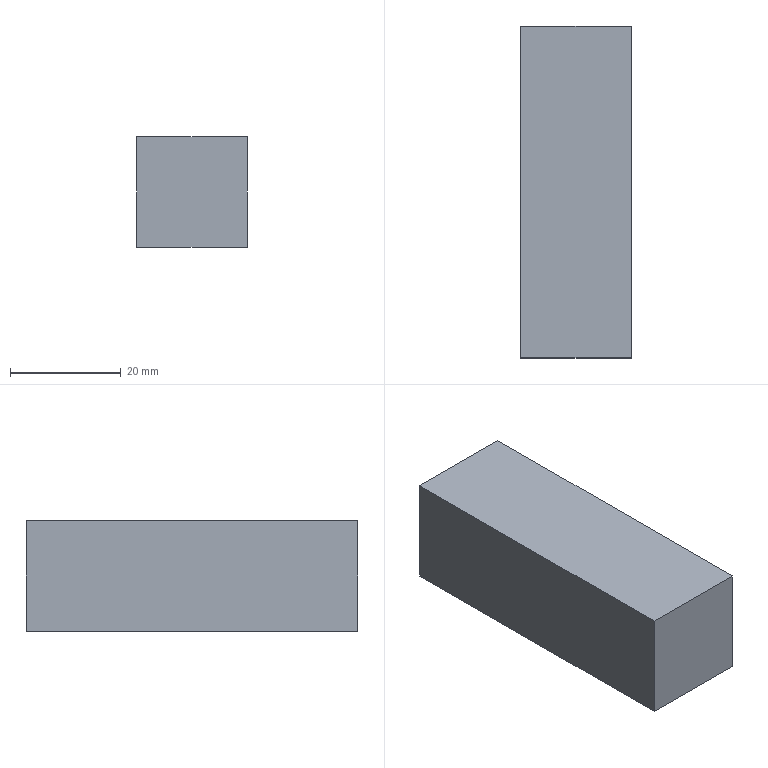Part | STEP file | 冲床-300配套压波_id186_x_t | 1 solid | 6 faces | box 20 x 60 x 20 mm | volume 24000 mm3 | plane 6
STEP:
#1=CARTESIAN_POINT('',(1125.,-215.,0.));
#2=VERTEX_POINT('',#1);
#3=CARTESIAN_POINT('',(1105.,-215.,0.));
#4=VERTEX_POINT('',#3);
#5=CARTESIAN_POINT('',(1105.,-215.,0.));
#6=DIRECTION('',(-1.,0.,0.));
#7=VECTOR('',#6,1.);
#8=LINE('',#5,#7);
#9=EDGE_CURVE('',#2,#4,#8,.T.);
#10=ORIENTED_EDGE('',*,*,#9,.F.);
#11=CARTESIAN_POINT('',(1125.,-155.,0.));
#12=VERTEX_POINT('',#11);
#13=CARTESIAN_POINT('',(1125.,-215.,0.));
#14=DIRECTION('',(0.,-1.,0.));
#15=VECTOR('',#14,1.);
#16=LINE('',#13,#15);
#17=EDGE_CURVE('',#12,#2,#16,.T.);
#18=ORIENTED_EDGE('',*,*,#17,.F.);
#19=CARTESIAN_POINT('',(1105.,-155.,0.));
#20=VERTEX_POINT('',#19);
#21=CARTESIAN_POINT('',(1105.,-155.,0.));
#22=DIRECTION('',(-1.,0.,0.));
#23=VECTOR('',#22,1.);
#24=LINE('',#21,#23);
#25=EDGE_CURVE('',#12,#20,#24,.T.);
#26=ORIENTED_EDGE('',*,*,#25,.T.);
#27=CARTESIAN_POINT('',(1105.,-215.,0.));
#28=DIRECTION('',(0.,-1.,0.));
#29=VECTOR('',#28,1.);
#30=LINE('',#27,#29);
#31=EDGE_CURVE('',#20,#4,#30,.T.);
#32=ORIENTED_EDGE('',*,*,#31,.T.);
#33=EDGE_LOOP('',(#10,#18,#26,#32));
#34=FACE_OUTER_BOUND('',#33,.T.);
#35=CARTESIAN_POINT('',(1105.,-215.,0.));
#36=DIRECTION('',(0.,0.,1.));
#37=DIRECTION('',(0.,1.,0.));
#38=AXIS2_PLACEMENT_3D('',#35,#36,#37);
#39=PLANE('',#38);
#40=ADVANCED_FACE('',(#34),#39,.T.);
#41=ORIENTED_EDGE('',*,*,#25,.F.);
#42=CARTESIAN_POINT('',(1125.,-155.,-20.));
#43=VERTEX_POINT('',#42);
#44=CARTESIAN_POINT('',(1125.,-155.,0.));
#45=DIRECTION('',(0.,0.,1.));
#46=VECTOR('',#45,1.);
#47=LINE('',#44,#46);
#48=EDGE_CURVE('',#43,#12,#47,.T.);
#49=ORIENTED_EDGE('',*,*,#48,.F.);
#50=CARTESIAN_POINT('',(1105.,-155.,-20.));
#51=VERTEX_POINT('',#50);
#52=CARTESIAN_POINT('',(1105.,-155.,-20.));
#53=DIRECTION('',(-1.,0.,0.));
#54=VECTOR('',#53,1.);
#55=LINE('',#52,#54);
#56=EDGE_CURVE('',#43,#51,#55,.T.);
#57=ORIENTED_EDGE('',*,*,#56,.T.);
#58=CARTESIAN_POINT('',(1105.,-155.,0.));
#59=DIRECTION('',(0.,0.,1.));
#60=VECTOR('',#59,1.);
#61=LINE('',#58,#60);
#62=EDGE_CURVE('',#51,#20,#61,.T.);
#63=ORIENTED_EDGE('',*,*,#62,.T.);
#64=EDGE_LOOP('',(#41,#49,#57,#63));
#65=FACE_OUTER_BOUND('',#64,.T.);
#66=CARTESIAN_POINT('',(1105.,-155.,0.));
#67=DIRECTION('',(0.,1.,0.));
#68=DIRECTION('',(0.,0.,-1.));
#69=AXIS2_PLACEMENT_3D('',#66,#67,#68);
#70=PLANE('',#69);
#71=ADVANCED_FACE('',(#65),#70,.T.);
#72=ORIENTED_EDGE('',*,*,#56,.F.);
#73=CARTESIAN_POINT('',(1125.,-215.,-20.));
#74=VERTEX_POINT('',#73);
#75=CARTESIAN_POINT('',(1125.,-215.,-20.));
#76=DIRECTION('',(0.,-1.,0.));
#77=VECTOR('',#76,1.);
#78=LINE('',#75,#77);
#79=EDGE_CURVE('',#43,#74,#78,.T.);
#80=ORIENTED_EDGE('',*,*,#79,.T.);
#81=CARTESIAN_POINT('',(1105.,-215.,-20.));
#82=VERTEX_POINT('',#81);
#83=CARTESIAN_POINT('',(1105.,-215.,-20.));
#84=DIRECTION('',(-1.,0.,0.));
#85=VECTOR('',#84,1.);
#86=LINE('',#83,#85);
#87=EDGE_CURVE('',#74,#82,#86,.T.);
#88=ORIENTED_EDGE('',*,*,#87,.T.);
#89=CARTESIAN_POINT('',(1105.,-215.,-20.));
#90=DIRECTION('',(0.,-1.,0.));
#91=VECTOR('',#90,1.);
#92=LINE('',#89,#91);
#93=EDGE_CURVE('',#51,#82,#92,.T.);
#94=ORIENTED_EDGE('',*,*,#93,.F.);
#95=EDGE_LOOP('',(#72,#80,#88,#94));
#96=FACE_OUTER_BOUND('',#95,.T.);
#97=CARTESIAN_POINT('',(1105.,-215.,-20.));
#98=DIRECTION('',(0.,0.,1.));
#99=DIRECTION('',(0.,1.,0.));
#100=AXIS2_PLACEMENT_3D('',#97,#98,#99);
#101=PLANE('',#100);
#102=ADVANCED_FACE('',(#96),#101,.F.);
#103=CARTESIAN_POINT('',(1105.,-215.,0.));
#104=DIRECTION('',(0.,0.,1.));
#105=VECTOR('',#104,1.);
#106=LINE('',#103,#105);
#107=EDGE_CURVE('',#82,#4,#106,.T.);
#108=ORIENTED_EDGE('',*,*,#107,.F.);
#109=ORIENTED_EDGE('',*,*,#87,.F.);
#110=CARTESIAN_POINT('',(1125.,-215.,0.));
#111=DIRECTION('',(0.,0.,1.));
#112=VECTOR('',#111,1.);
#113=LINE('',#110,#112);
#114=EDGE_CURVE('',#74,#2,#113,.T.);
#115=ORIENTED_EDGE('',*,*,#114,.T.);
#116=ORIENTED_EDGE('',*,*,#9,.T.);
#117=EDGE_LOOP('',(#108,#109,#115,#116));
#118=FACE_OUTER_BOUND('',#117,.T.);
#119=CARTESIAN_POINT('',(1105.,-215.,0.));
#120=DIRECTION('',(0.,1.,0.));
#121=DIRECTION('',(0.,0.,-1.));
#122=AXIS2_PLACEMENT_3D('',#119,#120,#121);
#123=PLANE('',#122);
#124=ADVANCED_FACE('',(#118),#123,.F.);
#125=ORIENTED_EDGE('',*,*,#79,.F.);
#126=ORIENTED_EDGE('',*,*,#48,.T.);
#127=ORIENTED_EDGE('',*,*,#17,.T.);
#128=ORIENTED_EDGE('',*,*,#114,.F.);
#129=EDGE_LOOP('',(#125,#126,#127,#128));
#130=FACE_OUTER_BOUND('',#129,.T.);
#131=CARTESIAN_POINT('',(1125.,-215.,0.));
#132=DIRECTION('',(1.,0.,0.));
#133=DIRECTION('',(0.,0.,-1.));
#134=AXIS2_PLACEMENT_3D('',#131,#132,#133);
#135=PLANE('',#134);
#136=ADVANCED_FACE('',(#130),#135,.T.);
#137=ORIENTED_EDGE('',*,*,#93,.T.);
#138=ORIENTED_EDGE('',*,*,#107,.T.);
#139=ORIENTED_EDGE('',*,*,#31,.F.);
#140=ORIENTED_EDGE('',*,*,#62,.F.);
#141=EDGE_LOOP('',(#137,#138,#139,#140));
#142=FACE_OUTER_BOUND('',#141,.T.);
#143=CARTESIAN_POINT('',(1105.,-215.,0.));
#144=DIRECTION('',(1.,0.,0.));
#145=DIRECTION('',(0.,0.,-1.));
#146=AXIS2_PLACEMENT_3D('',#143,#144,#145);
#147=PLANE('',#146);
#148=ADVANCED_FACE('',(#142),#147,.F.);
#149=CLOSED_SHELL('',(#40,#71,#102,#124,#136,#148));
#150=MANIFOLD_SOLID_BREP('',#149);
#151=(LENGTH_UNIT()NAMED_UNIT(*)SI_UNIT(.MILLI.,.METRE.));
#152=UNCERTAINTY_MEASURE_WITH_UNIT(LENGTH_MEASURE(0.00002),#151,'','');
#153=(NAMED_UNIT(*)PLANE_ANGLE_UNIT()SI_UNIT($,.RADIAN.));
#154=PLANE_ANGLE_MEASURE_WITH_UNIT(PLANE_ANGLE_MEASURE(0.01745),#153);
#155=DIMENSIONAL_EXPONENTS(0.,0.,0.,0.,0.,0.,0.);
#156=(CONVERSION_BASED_UNIT('DEGREE',#154)NAMED_UNIT(#155)PLANE_ANGLE_UNIT());
#157=(NAMED_UNIT(*)SI_UNIT($,.STERADIAN.)SOLID_ANGLE_UNIT());
#158=(GEOMETRIC_REPRESENTATION_CONTEXT(3)GLOBAL_UNCERTAINTY_ASSIGNED_CONTEXT((#152))GLOBAL_UNIT_ASSIGNED_CONTEXT((#151,#156,#157))REPRESENTATION_CONTEXT('',''));
#159=ADVANCED_BREP_SHAPE_REPRESENTATION('',(#150),#158);